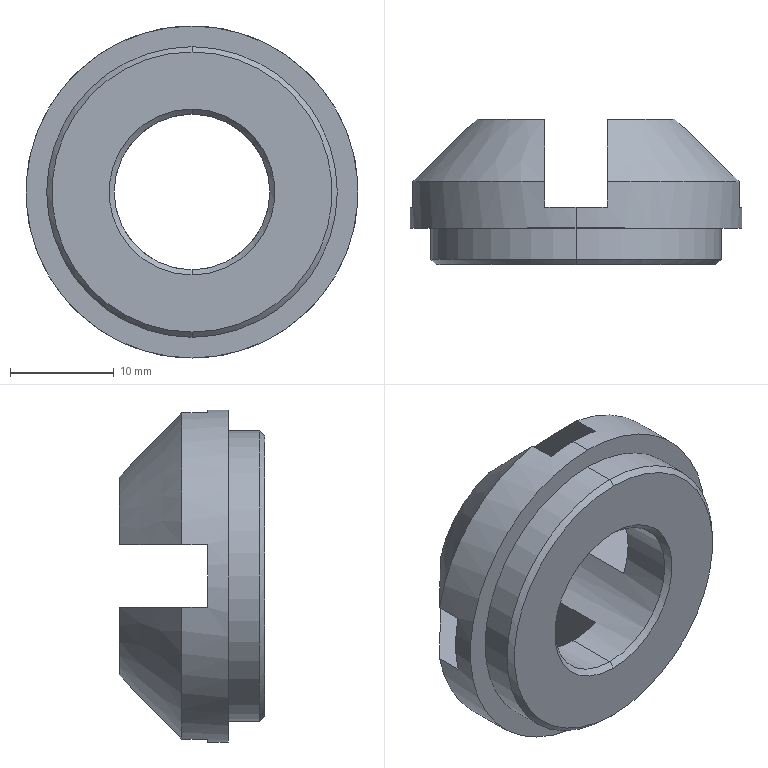Part | SolidWorks | features Chamfer 2, ICE 2, CirPattern 1, Revolution 1 | 1 solid | 32 faces | box 32 x 14 x 32 mm | volume 5204 mm3 | plane 18 | cone 8 | cylinder 6 | commonest cylinder face diameters 15 x2 28 x2 32 x2
STEP:
#1=CARTESIAN_POINT('',(0.,0.5,7.5));
#2=VERTEX_POINT('',#1);
#3=CARTESIAN_POINT('',(0.,0.5,-7.5));
#4=VERTEX_POINT('',#3);
#5=CARTESIAN_POINT('',(0.,0.5,0.));
#6=DIRECTION('',(0.,-1.,0.));
#7=DIRECTION('',(0.,0.,1.));
#8=AXIS2_PLACEMENT_3D('',#5,#6,#7);
#9=CIRCLE('',#8,7.5);
#10=EDGE_CURVE('',#2,#4,#9,.T.);
#11=ORIENTED_EDGE('',*,*,#10,.F.);
#12=CARTESIAN_POINT('',(0.,0.,8.));
#13=VERTEX_POINT('',#12);
#14=CARTESIAN_POINT('',(0.,0.,8.));
#15=DIRECTION('',(0.,-0.7071,0.7071));
#16=VECTOR('',#15,1000.);
#17=LINE('',#14,#16);
#18=EDGE_CURVE('',#2,#13,#17,.T.);
#19=ORIENTED_EDGE('',*,*,#18,.T.);
#20=CARTESIAN_POINT('',(0.,0.,-8.));
#21=VERTEX_POINT('',#20);
#22=CARTESIAN_POINT('',(0.,0.,0.));
#23=DIRECTION('',(0.,1.,0.));
#24=DIRECTION('',(0.,0.,1.));
#25=AXIS2_PLACEMENT_3D('',#22,#23,#24);
#26=CIRCLE('',#25,8.);
#27=EDGE_CURVE('',#21,#13,#26,.T.);
#28=ORIENTED_EDGE('',*,*,#27,.F.);
#29=CARTESIAN_POINT('',(0.,0.,-8.));
#30=DIRECTION('',(0.,-0.7071,-0.7071));
#31=VECTOR('',#30,1000.);
#32=LINE('',#29,#31);
#33=EDGE_CURVE('',#4,#21,#32,.T.);
#34=ORIENTED_EDGE('',*,*,#33,.F.);
#35=EDGE_LOOP('',(#11,#19,#28,#34));
#36=FACE_OUTER_BOUND('',#35,.T.);
#37=CARTESIAN_POINT('',(0.,0.,0.));
#38=DIRECTION('',(0.,-1.,0.));
#39=DIRECTION('',(0.,0.,-1.));
#40=AXIS2_PLACEMENT_3D('',#37,#38,#39);
#41=CONICAL_SURFACE('',#40,8.,0.7854);
#42=ADVANCED_FACE('',(#36),#41,.F.);
#43=CARTESIAN_POINT('',(0.,0.,-13.5));
#44=VERTEX_POINT('',#43);
#45=CARTESIAN_POINT('',(0.,0.,13.5));
#46=VERTEX_POINT('',#45);
#47=CARTESIAN_POINT('',(0.,0.,0.));
#48=DIRECTION('',(0.,-1.,0.));
#49=DIRECTION('',(0.,0.,1.));
#50=AXIS2_PLACEMENT_3D('',#47,#48,#49);
#51=CIRCLE('',#50,13.5);
#52=EDGE_CURVE('',#44,#46,#51,.T.);
#53=ORIENTED_EDGE('',*,*,#52,.F.);
#54=CARTESIAN_POINT('',(0.,0.5,-14.));
#55=VERTEX_POINT('',#54);
#56=CARTESIAN_POINT('',(0.,0.,-13.5));
#57=DIRECTION('',(0.,0.7071,-0.7071));
#58=VECTOR('',#57,1000.);
#59=LINE('',#56,#58);
#60=EDGE_CURVE('',#44,#55,#59,.T.);
#61=ORIENTED_EDGE('',*,*,#60,.T.);
#62=CARTESIAN_POINT('',(0.,0.5,14.));
#63=VERTEX_POINT('',#62);
#64=CARTESIAN_POINT('',(0.,0.5,0.));
#65=DIRECTION('',(0.,1.,0.));
#66=DIRECTION('',(0.,0.,1.));
#67=AXIS2_PLACEMENT_3D('',#64,#65,#66);
#68=CIRCLE('',#67,14.);
#69=EDGE_CURVE('',#63,#55,#68,.T.);
#70=ORIENTED_EDGE('',*,*,#69,.F.);
#71=CARTESIAN_POINT('',(0.,0.,13.5));
#72=DIRECTION('',(0.,0.7071,0.7071));
#73=VECTOR('',#72,1000.);
#74=LINE('',#71,#73);
#75=EDGE_CURVE('',#46,#63,#74,.T.);
#76=ORIENTED_EDGE('',*,*,#75,.F.);
#77=EDGE_LOOP('',(#53,#61,#70,#76));
#78=FACE_OUTER_BOUND('',#77,.T.);
#79=CARTESIAN_POINT('',(0.,0.,0.));
#80=DIRECTION('',(0.,1.,0.));
#81=DIRECTION('',(0.,0.,1.));
#82=AXIS2_PLACEMENT_3D('',#79,#80,#81);
#83=CONICAL_SURFACE('',#82,13.5,0.7854);
#84=ADVANCED_FACE('',(#78),#83,.T.);
#85=ORIENTED_EDGE('',*,*,#10,.T.);
#86=CARTESIAN_POINT('',(0.,5.5,-7.5));
#87=VERTEX_POINT('',#86);
#88=CARTESIAN_POINT('',(0.,-17.,-7.5));
#89=DIRECTION('',(0.,1.,0.));
#90=VECTOR('',#89,1000.);
#91=LINE('',#88,#90);
#92=EDGE_CURVE('',#4,#87,#91,.T.);
#93=ORIENTED_EDGE('',*,*,#92,.T.);
#94=CARTESIAN_POINT('',(-3.,5.5,-6.874));
#95=VERTEX_POINT('',#94);
#96=CARTESIAN_POINT('',(0.,5.5,0.));
#97=DIRECTION('',(0.,-1.,0.));
#98=DIRECTION('',(0.,0.,1.));
#99=AXIS2_PLACEMENT_3D('',#96,#97,#98);
#100=CIRCLE('',#99,7.5);
#101=EDGE_CURVE('',#95,#87,#100,.T.);
#102=ORIENTED_EDGE('',*,*,#101,.F.);
#103=CARTESIAN_POINT('',(-3.,14.,-6.874));
#104=VERTEX_POINT('',#103);
#105=CARTESIAN_POINT('',(-3.,-17.,-6.874));
#106=DIRECTION('',(0.,1.,0.));
#107=VECTOR('',#106,1000.);
#108=LINE('',#105,#107);
#109=EDGE_CURVE('',#95,#104,#108,.T.);
#110=ORIENTED_EDGE('',*,*,#109,.T.);
#111=CARTESIAN_POINT('',(-6.874,14.,-3.));
#112=VERTEX_POINT('',#111);
#113=CARTESIAN_POINT('',(0.,14.,0.));
#114=DIRECTION('',(0.,1.,0.));
#115=DIRECTION('',(0.,0.,1.));
#116=AXIS2_PLACEMENT_3D('',#113,#114,#115);
#117=CIRCLE('',#116,7.5);
#118=EDGE_CURVE('',#104,#112,#117,.T.);
#119=ORIENTED_EDGE('',*,*,#118,.T.);
#120=CARTESIAN_POINT('',(-6.874,5.5,-3.));
#121=VERTEX_POINT('',#120);
#122=CARTESIAN_POINT('',(-6.874,-17.,-3.));
#123=DIRECTION('',(0.,-1.,0.));
#124=VECTOR('',#123,1000.);
#125=LINE('',#122,#124);
#126=EDGE_CURVE('',#112,#121,#125,.T.);
#127=ORIENTED_EDGE('',*,*,#126,.T.);
#128=CARTESIAN_POINT('',(-6.874,5.5,3.));
#129=VERTEX_POINT('',#128);
#130=CARTESIAN_POINT('',(0.,5.5,0.));
#131=DIRECTION('',(0.,-1.,0.));
#132=DIRECTION('',(0.,0.,1.));
#133=AXIS2_PLACEMENT_3D('',#130,#131,#132);
#134=CIRCLE('',#133,7.5);
#135=EDGE_CURVE('',#129,#121,#134,.T.);
#136=ORIENTED_EDGE('',*,*,#135,.F.);
#137=CARTESIAN_POINT('',(-6.874,14.,3.));
#138=VERTEX_POINT('',#137);
#139=CARTESIAN_POINT('',(-6.874,-17.,3.));
#140=DIRECTION('',(0.,1.,0.));
#141=VECTOR('',#140,1000.);
#142=LINE('',#139,#141);
#143=EDGE_CURVE('',#129,#138,#142,.T.);
#144=ORIENTED_EDGE('',*,*,#143,.T.);
#145=CARTESIAN_POINT('',(-3.,14.,6.874));
#146=VERTEX_POINT('',#145);
#147=CARTESIAN_POINT('',(0.,14.,0.));
#148=DIRECTION('',(0.,1.,0.));
#149=DIRECTION('',(0.,0.,1.));
#150=AXIS2_PLACEMENT_3D('',#147,#148,#149);
#151=CIRCLE('',#150,7.5);
#152=EDGE_CURVE('',#138,#146,#151,.T.);
#153=ORIENTED_EDGE('',*,*,#152,.T.);
#154=CARTESIAN_POINT('',(-3.,5.5,6.874));
#155=VERTEX_POINT('',#154);
#156=CARTESIAN_POINT('',(-3.,-17.,6.874));
#157=DIRECTION('',(0.,-1.,0.));
#158=VECTOR('',#157,1000.);
#159=LINE('',#156,#158);
#160=EDGE_CURVE('',#146,#155,#159,.T.);
#161=ORIENTED_EDGE('',*,*,#160,.T.);
#162=CARTESIAN_POINT('',(0.,5.5,7.5));
#163=VERTEX_POINT('',#162);
#164=CARTESIAN_POINT('',(0.,5.5,0.));
#165=DIRECTION('',(0.,-1.,0.));
#166=DIRECTION('',(0.,0.,1.));
#167=AXIS2_PLACEMENT_3D('',#164,#165,#166);
#168=CIRCLE('',#167,7.5);
#169=EDGE_CURVE('',#163,#155,#168,.T.);
#170=ORIENTED_EDGE('',*,*,#169,.F.);
#171=CARTESIAN_POINT('',(0.,-17.,7.5));
#172=DIRECTION('',(0.,1.,0.));
#173=VECTOR('',#172,1000.);
#174=LINE('',#171,#173);
#175=EDGE_CURVE('',#2,#163,#174,.T.);
#176=ORIENTED_EDGE('',*,*,#175,.F.);
#177=EDGE_LOOP('',(#85,#93,#102,#110,#119,#127,#136,#144,#153,#161,#170,#176));
#178=FACE_OUTER_BOUND('',#177,.T.);
#179=CARTESIAN_POINT('',(0.,-17.,0.));
#180=DIRECTION('',(0.,1.,0.));
#181=DIRECTION('',(0.,0.,1.));
#182=AXIS2_PLACEMENT_3D('',#179,#180,#181);
#183=CYLINDRICAL_SURFACE('',#182,7.5);
#184=ADVANCED_FACE('',(#178),#183,.F.);
#185=CARTESIAN_POINT('',(0.,5.5,16.));
#186=VERTEX_POINT('',#185);
#187=CARTESIAN_POINT('',(3.,5.5,15.716));
#188=VERTEX_POINT('',#187);
#189=CARTESIAN_POINT('',(0.,5.5,0.));
#190=DIRECTION('',(0.,1.,0.));
#191=DIRECTION('',(0.,0.,1.));
#192=AXIS2_PLACEMENT_3D('',#189,#190,#191);
#193=CIRCLE('',#192,16.);
#194=EDGE_CURVE('',#186,#188,#193,.T.);
#195=ORIENTED_EDGE('',*,*,#194,.F.);
#196=CARTESIAN_POINT('',(0.,3.5,16.));
#197=VERTEX_POINT('',#196);
#198=CARTESIAN_POINT('',(0.,0.,16.));
#199=DIRECTION('',(0.,-1.,0.));
#200=VECTOR('',#199,1000.);
#201=LINE('',#198,#200);
#202=EDGE_CURVE('',#186,#197,#201,.T.);
#203=ORIENTED_EDGE('',*,*,#202,.T.);
#204=CARTESIAN_POINT('',(0.,3.5,-16.));
#205=VERTEX_POINT('',#204);
#206=CARTESIAN_POINT('',(0.,3.5,0.));
#207=DIRECTION('',(0.,-1.,0.));
#208=DIRECTION('',(0.,0.,-1.));
#209=AXIS2_PLACEMENT_3D('',#206,#207,#208);
#210=CIRCLE('',#209,16.);
#211=EDGE_CURVE('',#205,#197,#210,.T.);
#212=ORIENTED_EDGE('',*,*,#211,.F.);
#213=CARTESIAN_POINT('',(0.,5.5,-16.));
#214=VERTEX_POINT('',#213);
#215=CARTESIAN_POINT('',(0.,0.,-16.));
#216=DIRECTION('',(0.,-1.,0.));
#217=VECTOR('',#216,1000.);
#218=LINE('',#215,#217);
#219=EDGE_CURVE('',#214,#205,#218,.T.);
#220=ORIENTED_EDGE('',*,*,#219,.F.);
#221=CARTESIAN_POINT('',(3.,5.5,-15.716));
#222=VERTEX_POINT('',#221);
#223=CARTESIAN_POINT('',(0.,5.5,0.));
#224=DIRECTION('',(0.,1.,0.));
#225=DIRECTION('',(0.,0.,1.));
#226=AXIS2_PLACEMENT_3D('',#223,#224,#225);
#227=CIRCLE('',#226,16.);
#228=EDGE_CURVE('',#222,#214,#227,.T.);
#229=ORIENTED_EDGE('',*,*,#228,.F.);
#230=CARTESIAN_POINT('',(3.,8.,-15.716));
#231=VERTEX_POINT('',#230);
#232=CARTESIAN_POINT('',(3.,0.,-15.716));
#233=DIRECTION('',(0.,1.,0.));
#234=VECTOR('',#233,1000.);
#235=LINE('',#232,#234);
#236=EDGE_CURVE('',#222,#231,#235,.T.);
#237=ORIENTED_EDGE('',*,*,#236,.T.);
#238=CARTESIAN_POINT('',(15.716,8.,-3.));
#239=VERTEX_POINT('',#238);
#240=CARTESIAN_POINT('',(0.,8.,0.));
#241=DIRECTION('',(0.,-1.,0.));
#242=DIRECTION('',(0.,0.,-1.));
#243=AXIS2_PLACEMENT_3D('',#240,#241,#242);
#244=CIRCLE('',#243,16.);
#245=EDGE_CURVE('',#231,#239,#244,.T.);
#246=ORIENTED_EDGE('',*,*,#245,.T.);
#247=CARTESIAN_POINT('',(15.716,5.5,-3.));
#248=VERTEX_POINT('',#247);
#249=CARTESIAN_POINT('',(15.716,0.,-3.));
#250=DIRECTION('',(0.,-1.,0.));
#251=VECTOR('',#250,1000.);
#252=LINE('',#249,#251);
#253=EDGE_CURVE('',#239,#248,#252,.T.);
#254=ORIENTED_EDGE('',*,*,#253,.T.);
#255=CARTESIAN_POINT('',(15.716,5.5,3.));
#256=VERTEX_POINT('',#255);
#257=CARTESIAN_POINT('',(0.,5.5,0.));
#258=DIRECTION('',(0.,1.,0.));
#259=DIRECTION('',(0.,0.,1.));
#260=AXIS2_PLACEMENT_3D('',#257,#258,#259);
#261=CIRCLE('',#260,16.);
#262=EDGE_CURVE('',#256,#248,#261,.T.);
#263=ORIENTED_EDGE('',*,*,#262,.F.);
#264=CARTESIAN_POINT('',(15.716,8.,3.));
#265=VERTEX_POINT('',#264);
#266=CARTESIAN_POINT('',(15.716,0.,3.));
#267=DIRECTION('',(0.,1.,0.));
#268=VECTOR('',#267,1000.);
#269=LINE('',#266,#268);
#270=EDGE_CURVE('',#256,#265,#269,.T.);
#271=ORIENTED_EDGE('',*,*,#270,.T.);
#272=CARTESIAN_POINT('',(3.,8.,15.716));
#273=VERTEX_POINT('',#272);
#274=CARTESIAN_POINT('',(0.,8.,0.));
#275=DIRECTION('',(0.,-1.,0.));
#276=DIRECTION('',(0.,0.,-1.));
#277=AXIS2_PLACEMENT_3D('',#274,#275,#276);
#278=CIRCLE('',#277,16.);
#279=EDGE_CURVE('',#265,#273,#278,.T.);
#280=ORIENTED_EDGE('',*,*,#279,.T.);
#281=CARTESIAN_POINT('',(3.,0.,15.716));
#282=DIRECTION('',(0.,-1.,0.));
#283=VECTOR('',#282,1000.);
#284=LINE('',#281,#283);
#285=EDGE_CURVE('',#273,#188,#284,.T.);
#286=ORIENTED_EDGE('',*,*,#285,.T.);
#287=EDGE_LOOP('',(#195,#203,#212,#220,#229,#237,#246,#254,#263,#271,#280,#286));
#288=FACE_OUTER_BOUND('',#287,.T.);
#289=CARTESIAN_POINT('',(0.,0.,0.));
#290=DIRECTION('',(0.,-1.,0.));
#291=DIRECTION('',(0.,0.,-1.));
#292=AXIS2_PLACEMENT_3D('',#289,#290,#291);
#293=CYLINDRICAL_SURFACE('',#292,16.);
#294=ADVANCED_FACE('',(#288),#293,.T.);
#295=CARTESIAN_POINT('',(0.,3.5,-14.));
#296=VERTEX_POINT('',#295);
#297=CARTESIAN_POINT('',(0.,3.5,14.));
#298=VERTEX_POINT('',#297);
#299=CARTESIAN_POINT('',(0.,3.5,0.));
#300=DIRECTION('',(0.,-1.,0.));
#301=DIRECTION('',(0.,0.,-1.));
#302=AXIS2_PLACEMENT_3D('',#299,#300,#301);
#303=CIRCLE('',#302,14.);
#304=EDGE_CURVE('',#296,#298,#303,.T.);
#305=ORIENTED_EDGE('',*,*,#304,.T.);
#306=CARTESIAN_POINT('',(0.,0.,14.));
#307=DIRECTION('',(0.,-1.,0.));
#308=VECTOR('',#307,1000.);
#309=LINE('',#306,#308);
#310=EDGE_CURVE('',#298,#63,#309,.T.);
#311=ORIENTED_EDGE('',*,*,#310,.T.);
#312=ORIENTED_EDGE('',*,*,#69,.T.);
#313=CARTESIAN_POINT('',(0.,0.,-14.));
#314=DIRECTION('',(0.,-1.,0.));
#315=VECTOR('',#314,1000.);
#316=LINE('',#313,#315);
#317=EDGE_CURVE('',#296,#55,#316,.T.);
#318=ORIENTED_EDGE('',*,*,#317,.F.);
#319=EDGE_LOOP('',(#305,#311,#312,#318));
#320=FACE_OUTER_BOUND('',#319,.T.);
#321=CARTESIAN_POINT('',(0.,0.,0.));
#322=DIRECTION('',(0.,-1.,0.));
#323=DIRECTION('',(0.,0.,-1.));
#324=AXIS2_PLACEMENT_3D('',#321,#322,#323);
#325=CYLINDRICAL_SURFACE('',#324,14.);
#326=ADVANCED_FACE('',(#320),#325,.T.);
#327=CARTESIAN_POINT('',(9.539,14.,3.));
#328=VERTEX_POINT('',#327);
#329=CARTESIAN_POINT('',(3.,14.,9.539));
#330=VERTEX_POINT('',#329);
#331=CARTESIAN_POINT('',(0.,14.,0.));
#332=DIRECTION('',(0.,-1.,0.));
#333=DIRECTION('',(0.,0.,-1.));
#334=AXIS2_PLACEMENT_3D('',#331,#332,#333);
#335=CIRCLE('',#334,10.);
#336=EDGE_CURVE('',#328,#330,#335,.T.);
#337=ORIENTED_EDGE('',*,*,#336,.T.);
#338=CARTESIAN_POINT('',(3.,14.,9.539));
#339=CARTESIAN_POINT('',(3.,12.019,11.616));
#340=CARTESIAN_POINT('',(3.,10.012,13.668));
#341=CARTESIAN_POINT('',(3.,8.,15.716));
#342=B_SPLINE_CURVE_WITH_KNOTS('',3,(#338,#339,#340,#341),.UNSPECIFIED.,.F.,.F.,(4,4),(0.01205,0.02069),.UNSPECIFIED.);
#343=EDGE_CURVE('',#330,#273,#342,.T.);
#344=ORIENTED_EDGE('',*,*,#343,.T.);
#345=ORIENTED_EDGE('',*,*,#279,.F.);
#346=CARTESIAN_POINT('',(15.716,8.,3.));
#347=CARTESIAN_POINT('',(13.668,10.012,3.));
#348=CARTESIAN_POINT('',(11.616,12.019,3.));
#349=CARTESIAN_POINT('',(9.539,14.,3.));
#350=B_SPLINE_CURVE_WITH_KNOTS('',3,(#346,#347,#348,#349),.UNSPECIFIED.,.F.,.F.,(4,4),(0.000000998,0.008605),.UNSPECIFIED.);
#351=EDGE_CURVE('',#265,#328,#350,.T.);
#352=ORIENTED_EDGE('',*,*,#351,.T.);
#353=EDGE_LOOP('',(#337,#344,#345,#352));
#354=FACE_OUTER_BOUND('',#353,.T.);
#355=CARTESIAN_POINT('',(0.,14.,0.));
#356=DIRECTION('',(0.,-1.,0.));
#357=DIRECTION('',(0.,0.,-1.));
#358=AXIS2_PLACEMENT_3D('',#355,#356,#357);
#359=CONICAL_SURFACE('',#358,10.,0.7854);
#360=ADVANCED_FACE('',(#354),#359,.T.);
#361=CARTESIAN_POINT('',(3.,14.,6.874));
#362=VERTEX_POINT('',#361);
#363=CARTESIAN_POINT('',(6.874,14.,3.));
#364=VERTEX_POINT('',#363);
#365=CARTESIAN_POINT('',(0.,14.,0.));
#366=DIRECTION('',(0.,1.,0.));
#367=DIRECTION('',(0.,0.,1.));
#368=AXIS2_PLACEMENT_3D('',#365,#366,#367);
#369=CIRCLE('',#368,7.5);
#370=EDGE_CURVE('',#362,#364,#369,.T.);
#371=ORIENTED_EDGE('',*,*,#370,.F.);
#372=CARTESIAN_POINT('',(3.,14.,20.34));
#373=DIRECTION('',(0.,0.,-1.));
#374=VECTOR('',#373,1000.);
#375=LINE('',#372,#374);
#376=EDGE_CURVE('',#330,#362,#375,.T.);
#377=ORIENTED_EDGE('',*,*,#376,.F.);
#378=ORIENTED_EDGE('',*,*,#336,.F.);
#379=CARTESIAN_POINT('',(-20.34,14.,3.));
#380=DIRECTION('',(1.,0.,0.));
#381=VECTOR('',#380,1000.);
#382=LINE('',#379,#381);
#383=EDGE_CURVE('',#364,#328,#382,.T.);
#384=ORIENTED_EDGE('',*,*,#383,.F.);
#385=EDGE_LOOP('',(#371,#377,#378,#384));
#386=FACE_OUTER_BOUND('',#385,.T.);
#387=CARTESIAN_POINT('',(-10.,14.,0.));
#388=DIRECTION('',(0.,-1.,0.));
#389=DIRECTION('',(0.,0.,-1.));
#390=AXIS2_PLACEMENT_3D('',#387,#388,#389);
#391=PLANE('',#390);
#392=ADVANCED_FACE('',(#386),#391,.F.);
#393=ORIENTED_EDGE('',*,*,#245,.F.);
#394=CARTESIAN_POINT('',(3.,14.,-9.539));
#395=VERTEX_POINT('',#394);
#396=CARTESIAN_POINT('',(3.,8.,-15.716));
#397=CARTESIAN_POINT('',(3.,10.011,-13.668));
#398=CARTESIAN_POINT('',(3.,12.019,-11.616));
#399=CARTESIAN_POINT('',(3.,14.,-9.539));
#400=B_SPLINE_CURVE_WITH_KNOTS('',3,(#396,#397,#398,#399),.UNSPECIFIED.,.F.,.F.,(4,4),(0.000000999,0.008612),.UNSPECIFIED.);
#401=EDGE_CURVE('',#231,#395,#400,.T.);
#402=ORIENTED_EDGE('',*,*,#401,.T.);
#403=CARTESIAN_POINT('',(9.539,14.,-3.));
#404=VERTEX_POINT('',#403);
#405=CARTESIAN_POINT('',(0.,14.,0.));
#406=DIRECTION('',(0.,-1.,0.));
#407=DIRECTION('',(0.,0.,-1.));
#408=AXIS2_PLACEMENT_3D('',#405,#406,#407);
#409=CIRCLE('',#408,10.);
#410=EDGE_CURVE('',#395,#404,#409,.T.);
#411=ORIENTED_EDGE('',*,*,#410,.T.);
#412=CARTESIAN_POINT('',(9.539,14.,-3.));
#413=CARTESIAN_POINT('',(11.616,12.019,-3.));
#414=CARTESIAN_POINT('',(13.668,10.012,-3.));
#415=CARTESIAN_POINT('',(15.716,8.,-3.));
#416=B_SPLINE_CURVE_WITH_KNOTS('',3,(#412,#413,#414,#415),.UNSPECIFIED.,.F.,.F.,(4,4),(0.03228,0.0407),.UNSPECIFIED.);
#417=EDGE_CURVE('',#404,#239,#416,.T.);
#418=ORIENTED_EDGE('',*,*,#417,.T.);
#419=EDGE_LOOP('',(#393,#402,#411,#418));
#420=FACE_OUTER_BOUND('',#419,.T.);
#421=CARTESIAN_POINT('',(0.,14.,0.));
#422=DIRECTION('',(0.,-1.,0.));
#423=DIRECTION('',(0.,0.,-1.));
#424=AXIS2_PLACEMENT_3D('',#421,#422,#423);
#425=CONICAL_SURFACE('',#424,10.,0.7854);
#426=ADVANCED_FACE('',(#420),#425,.T.);
#427=ORIENTED_EDGE('',*,*,#410,.F.);
#428=CARTESIAN_POINT('',(3.,14.,-6.874));
#429=VERTEX_POINT('',#428);
#430=CARTESIAN_POINT('',(3.,14.,20.34));
#431=DIRECTION('',(0.,0.,-1.));
#432=VECTOR('',#431,1000.);
#433=LINE('',#430,#432);
#434=EDGE_CURVE('',#429,#395,#433,.T.);
#435=ORIENTED_EDGE('',*,*,#434,.F.);
#436=CARTESIAN_POINT('',(6.874,14.,-3.));
#437=VERTEX_POINT('',#436);
#438=CARTESIAN_POINT('',(0.,14.,0.));
#439=DIRECTION('',(0.,1.,0.));
#440=DIRECTION('',(0.,0.,1.));
#441=AXIS2_PLACEMENT_3D('',#438,#439,#440);
#442=CIRCLE('',#441,7.5);
#443=EDGE_CURVE('',#437,#429,#442,.T.);
#444=ORIENTED_EDGE('',*,*,#443,.F.);
#445=CARTESIAN_POINT('',(-20.34,14.,-3.));
#446=DIRECTION('',(-1.,0.,0.));
#447=VECTOR('',#446,1000.);
#448=LINE('',#445,#447);
#449=EDGE_CURVE('',#404,#437,#448,.T.);
#450=ORIENTED_EDGE('',*,*,#449,.F.);
#451=EDGE_LOOP('',(#427,#435,#444,#450));
#452=FACE_OUTER_BOUND('',#451,.T.);
#453=CARTESIAN_POINT('',(-10.,14.,0.));
#454=DIRECTION('',(0.,-1.,0.));
#455=DIRECTION('',(0.,0.,-1.));
#456=AXIS2_PLACEMENT_3D('',#453,#454,#455);
#457=PLANE('',#456);
#458=ADVANCED_FACE('',(#452),#457,.F.);
#459=CARTESIAN_POINT('',(-3.,8.,15.716));
#460=VERTEX_POINT('',#459);
#461=CARTESIAN_POINT('',(-15.716,8.,3.));
#462=VERTEX_POINT('',#461);
#463=CARTESIAN_POINT('',(0.,8.,0.));
#464=DIRECTION('',(0.,-1.,0.));
#465=DIRECTION('',(0.,0.,-1.));
#466=AXIS2_PLACEMENT_3D('',#463,#464,#465);
#467=CIRCLE('',#466,16.);
#468=EDGE_CURVE('',#460,#462,#467,.T.);
#469=ORIENTED_EDGE('',*,*,#468,.F.);
#470=CARTESIAN_POINT('',(-3.,14.,9.539));
#471=VERTEX_POINT('',#470);
#472=CARTESIAN_POINT('',(-3.,8.,15.716));
#473=CARTESIAN_POINT('',(-3.,10.011,13.668));
#474=CARTESIAN_POINT('',(-3.,12.019,11.616));
#475=CARTESIAN_POINT('',(-3.,14.,9.539));
#476=B_SPLINE_CURVE_WITH_KNOTS('',3,(#472,#473,#474,#475),.UNSPECIFIED.,.F.,.F.,(4,4),(0.000000999,0.008612),.UNSPECIFIED.);
#477=EDGE_CURVE('',#460,#471,#476,.T.);
#478=ORIENTED_EDGE('',*,*,#477,.T.);
#479=CARTESIAN_POINT('',(-9.539,14.,3.));
#480=VERTEX_POINT('',#479);
#481=CARTESIAN_POINT('',(0.,14.,0.));
#482=DIRECTION('',(0.,-1.,0.));
#483=DIRECTION('',(0.,0.,-1.));
#484=AXIS2_PLACEMENT_3D('',#481,#482,#483);
#485=CIRCLE('',#484,10.);
#486=EDGE_CURVE('',#471,#480,#485,.T.);
#487=ORIENTED_EDGE('',*,*,#486,.T.);
#488=CARTESIAN_POINT('',(-9.539,14.,3.));
#489=CARTESIAN_POINT('',(-11.616,12.019,3.));
#490=CARTESIAN_POINT('',(-13.668,10.012,3.));
#491=CARTESIAN_POINT('',(-15.716,8.,3.));
#492=B_SPLINE_CURVE_WITH_KNOTS('',3,(#488,#489,#490,#491),.UNSPECIFIED.,.F.,.F.,(4,4),(0.03228,0.0407),.UNSPECIFIED.);
#493=EDGE_CURVE('',#480,#462,#492,.T.);
#494=ORIENTED_EDGE('',*,*,#493,.T.);
#495=EDGE_LOOP('',(#469,#478,#487,#494));
#496=FACE_OUTER_BOUND('',#495,.T.);
#497=CARTESIAN_POINT('',(0.,14.,0.));
#498=DIRECTION('',(0.,-1.,0.));
#499=DIRECTION('',(0.,0.,-1.));
#500=AXIS2_PLACEMENT_3D('',#497,#498,#499);
#501=CONICAL_SURFACE('',#500,10.,0.7854);
#502=ADVANCED_FACE('',(#496),#501,.T.);
#503=ORIENTED_EDGE('',*,*,#486,.F.);
#504=CARTESIAN_POINT('',(-3.,14.,20.34));
#505=DIRECTION('',(0.,0.,1.));
#506=VECTOR('',#505,1000.);
#507=LINE('',#504,#506);
#508=EDGE_CURVE('',#146,#471,#507,.T.);
#509=ORIENTED_EDGE('',*,*,#508,.F.);
#510=ORIENTED_EDGE('',*,*,#152,.F.);
#511=CARTESIAN_POINT('',(-20.34,14.,3.));
#512=DIRECTION('',(1.,0.,0.));
#513=VECTOR('',#512,1000.);
#514=LINE('',#511,#513);
#515=EDGE_CURVE('',#480,#138,#514,.T.);
#516=ORIENTED_EDGE('',*,*,#515,.F.);
#517=EDGE_LOOP('',(#503,#509,#510,#516));
#518=FACE_OUTER_BOUND('',#517,.T.);
#519=CARTESIAN_POINT('',(-10.,14.,0.));
#520=DIRECTION('',(0.,-1.,0.));
#521=DIRECTION('',(0.,0.,-1.));
#522=AXIS2_PLACEMENT_3D('',#519,#520,#521);
#523=PLANE('',#522);
#524=ADVANCED_FACE('',(#518),#523,.F.);
#525=ORIENTED_EDGE('',*,*,#27,.T.);
#526=CARTESIAN_POINT('',(0.,0.,0.));
#527=DIRECTION('',(0.,1.,0.));
#528=DIRECTION('',(0.,0.,1.));
#529=AXIS2_PLACEMENT_3D('',#526,#527,#528);
#530=CIRCLE('',#529,8.);
#531=EDGE_CURVE('',#13,#21,#530,.T.);
#532=ORIENTED_EDGE('',*,*,#531,.T.);
#533=EDGE_LOOP('',(#525,#532));
#534=FACE_BOUND('',#533,.T.);
#535=CARTESIAN_POINT('',(0.,0.,0.));
#536=DIRECTION('',(0.,-1.,0.));
#537=DIRECTION('',(0.,0.,1.));
#538=AXIS2_PLACEMENT_3D('',#535,#536,#537);
#539=CIRCLE('',#538,13.5);
#540=EDGE_CURVE('',#46,#44,#539,.T.);
#541=ORIENTED_EDGE('',*,*,#540,.T.);
#542=ORIENTED_EDGE('',*,*,#52,.T.);
#543=EDGE_LOOP('',(#541,#542));
#544=FACE_OUTER_BOUND('',#543,.T.);
#545=CARTESIAN_POINT('',(0.,0.,0.));
#546=DIRECTION('',(0.,1.,0.));
#547=DIRECTION('',(0.,0.,1.));
#548=AXIS2_PLACEMENT_3D('',#545,#546,#547);
#549=PLANE('',#548);
#550=ADVANCED_FACE('',(#534,#544),#549,.F.);
#551=ORIENTED_EDGE('',*,*,#310,.F.);
#552=CARTESIAN_POINT('',(0.,3.5,0.));
#553=DIRECTION('',(0.,-1.,0.));
#554=DIRECTION('',(0.,0.,-1.));
#555=AXIS2_PLACEMENT_3D('',#552,#553,#554);
#556=CIRCLE('',#555,14.);
#557=EDGE_CURVE('',#298,#296,#556,.T.);
#558=ORIENTED_EDGE('',*,*,#557,.T.);
#559=ORIENTED_EDGE('',*,*,#317,.T.);
#560=CARTESIAN_POINT('',(0.,0.5,0.));
#561=DIRECTION('',(0.,1.,0.));
#562=DIRECTION('',(0.,0.,1.));
#563=AXIS2_PLACEMENT_3D('',#560,#561,#562);
#564=CIRCLE('',#563,14.);
#565=EDGE_CURVE('',#55,#63,#564,.T.);
#566=ORIENTED_EDGE('',*,*,#565,.T.);
#567=EDGE_LOOP('',(#551,#558,#559,#566));
#568=FACE_OUTER_BOUND('',#567,.T.);
#569=CARTESIAN_POINT('',(0.,0.,0.));
#570=DIRECTION('',(0.,-1.,0.));
#571=DIRECTION('',(0.,0.,-1.));
#572=AXIS2_PLACEMENT_3D('',#569,#570,#571);
#573=CYLINDRICAL_SURFACE('',#572,14.);
#574=ADVANCED_FACE('',(#568),#573,.T.);
#575=ORIENTED_EDGE('',*,*,#304,.F.);
#576=ORIENTED_EDGE('',*,*,#557,.F.);
#577=EDGE_LOOP('',(#575,#576));
#578=FACE_BOUND('',#577,.T.);
#579=ORIENTED_EDGE('',*,*,#211,.T.);
#580=CARTESIAN_POINT('',(0.,3.5,0.));
#581=DIRECTION('',(0.,-1.,0.));
#582=DIRECTION('',(0.,0.,-1.));
#583=AXIS2_PLACEMENT_3D('',#580,#581,#582);
#584=CIRCLE('',#583,16.);
#585=EDGE_CURVE('',#197,#205,#584,.T.);
#586=ORIENTED_EDGE('',*,*,#585,.T.);
#587=EDGE_LOOP('',(#579,#586));
#588=FACE_OUTER_BOUND('',#587,.T.);
#589=CARTESIAN_POINT('',(-14.,3.5,0.));
#590=DIRECTION('',(0.,1.,0.));
#591=DIRECTION('',(0.,0.,1.));
#592=AXIS2_PLACEMENT_3D('',#589,#590,#591);
#593=PLANE('',#592);
#594=ADVANCED_FACE('',(#578,#588),#593,.F.);
#595=ORIENTED_EDGE('',*,*,#202,.F.);
#596=CARTESIAN_POINT('',(-3.,5.5,15.716));
#597=VERTEX_POINT('',#596);
#598=CARTESIAN_POINT('',(0.,5.5,0.));
#599=DIRECTION('',(0.,1.,0.));
#600=DIRECTION('',(0.,0.,1.));
#601=AXIS2_PLACEMENT_3D('',#598,#599,#600);
#602=CIRCLE('',#601,16.);
#603=EDGE_CURVE('',#597,#186,#602,.T.);
#604=ORIENTED_EDGE('',*,*,#603,.F.);
#605=CARTESIAN_POINT('',(-3.,0.,15.716));
#606=DIRECTION('',(0.,1.,0.));
#607=VECTOR('',#606,1000.);
#608=LINE('',#605,#607);
#609=EDGE_CURVE('',#597,#460,#608,.T.);
#610=ORIENTED_EDGE('',*,*,#609,.T.);
#611=ORIENTED_EDGE('',*,*,#468,.T.);
#612=CARTESIAN_POINT('',(-15.716,5.5,3.));
#613=VERTEX_POINT('',#612);
#614=CARTESIAN_POINT('',(-15.716,0.,3.));
#615=DIRECTION('',(0.,-1.,0.));
#616=VECTOR('',#615,1000.);
#617=LINE('',#614,#616);
#618=EDGE_CURVE('',#462,#613,#617,.T.);
#619=ORIENTED_EDGE('',*,*,#618,.T.);
#620=CARTESIAN_POINT('',(-15.716,5.5,-3.));
#621=VERTEX_POINT('',#620);
#622=CARTESIAN_POINT('',(0.,5.5,0.));
#623=DIRECTION('',(0.,1.,0.));
#624=DIRECTION('',(0.,0.,1.));
#625=AXIS2_PLACEMENT_3D('',#622,#623,#624);
#626=CIRCLE('',#625,16.);
#627=EDGE_CURVE('',#621,#613,#626,.T.);
#628=ORIENTED_EDGE('',*,*,#627,.F.);
#629=CARTESIAN_POINT('',(-15.716,8.,-3.));
#630=VERTEX_POINT('',#629);
#631=CARTESIAN_POINT('',(-15.716,0.,-3.));
#632=DIRECTION('',(0.,1.,0.));
#633=VECTOR('',#632,1000.);
#634=LINE('',#631,#633);
#635=EDGE_CURVE('',#621,#630,#634,.T.);
#636=ORIENTED_EDGE('',*,*,#635,.T.);
#637=CARTESIAN_POINT('',(-3.,8.,-15.716));
#638=VERTEX_POINT('',#637);
#639=CARTESIAN_POINT('',(0.,8.,0.));
#640=DIRECTION('',(0.,-1.,0.));
#641=DIRECTION('',(0.,0.,-1.));
#642=AXIS2_PLACEMENT_3D('',#639,#640,#641);
#643=CIRCLE('',#642,16.);
#644=EDGE_CURVE('',#630,#638,#643,.T.);
#645=ORIENTED_EDGE('',*,*,#644,.T.);
#646=CARTESIAN_POINT('',(-3.,5.5,-15.716));
#647=VERTEX_POINT('',#646);
#648=CARTESIAN_POINT('',(-3.,0.,-15.716));
#649=DIRECTION('',(0.,-1.,0.));
#650=VECTOR('',#649,1000.);
#651=LINE('',#648,#650);
#652=EDGE_CURVE('',#638,#647,#651,.T.);
#653=ORIENTED_EDGE('',*,*,#652,.T.);
#654=CARTESIAN_POINT('',(0.,5.5,0.));
#655=DIRECTION('',(0.,1.,0.));
#656=DIRECTION('',(0.,0.,1.));
#657=AXIS2_PLACEMENT_3D('',#654,#655,#656);
#658=CIRCLE('',#657,16.);
#659=EDGE_CURVE('',#214,#647,#658,.T.);
#660=ORIENTED_EDGE('',*,*,#659,.F.);
#661=ORIENTED_EDGE('',*,*,#219,.T.);
#662=ORIENTED_EDGE('',*,*,#585,.F.);
#663=EDGE_LOOP('',(#595,#604,#610,#611,#619,#628,#636,#645,#653,#660,#661,#662));
#664=FACE_OUTER_BOUND('',#663,.T.);
#665=CARTESIAN_POINT('',(0.,0.,0.));
#666=DIRECTION('',(0.,-1.,0.));
#667=DIRECTION('',(0.,0.,-1.));
#668=AXIS2_PLACEMENT_3D('',#665,#666,#667);
#669=CYLINDRICAL_SURFACE('',#668,16.);
#670=ADVANCED_FACE('',(#664),#669,.T.);
#671=CARTESIAN_POINT('',(-9.539,14.,-3.));
#672=VERTEX_POINT('',#671);
#673=CARTESIAN_POINT('',(-3.,14.,-9.539));
#674=VERTEX_POINT('',#673);
#675=CARTESIAN_POINT('',(0.,14.,0.));
#676=DIRECTION('',(0.,-1.,0.));
#677=DIRECTION('',(0.,0.,-1.));
#678=AXIS2_PLACEMENT_3D('',#675,#676,#677);
#679=CIRCLE('',#678,10.);
#680=EDGE_CURVE('',#672,#674,#679,.T.);
#681=ORIENTED_EDGE('',*,*,#680,.T.);
#682=CARTESIAN_POINT('',(-3.,14.,-9.539));
#683=CARTESIAN_POINT('',(-3.,12.019,-11.616));
#684=CARTESIAN_POINT('',(-3.,10.012,-13.668));
#685=CARTESIAN_POINT('',(-3.,8.,-15.716));
#686=B_SPLINE_CURVE_WITH_KNOTS('',3,(#682,#683,#684,#685),.UNSPECIFIED.,.F.,.F.,(4,4),(0.01205,0.02069),.UNSPECIFIED.);
#687=EDGE_CURVE('',#674,#638,#686,.T.);
#688=ORIENTED_EDGE('',*,*,#687,.T.);
#689=ORIENTED_EDGE('',*,*,#644,.F.);
#690=CARTESIAN_POINT('',(-15.716,8.,-3.));
#691=CARTESIAN_POINT('',(-13.668,10.012,-3.));
#692=CARTESIAN_POINT('',(-11.616,12.019,-3.));
#693=CARTESIAN_POINT('',(-9.539,14.,-3.));
#694=B_SPLINE_CURVE_WITH_KNOTS('',3,(#690,#691,#692,#693),.UNSPECIFIED.,.F.,.F.,(4,4),(0.000000998,0.008605),.UNSPECIFIED.);
#695=EDGE_CURVE('',#630,#672,#694,.T.);
#696=ORIENTED_EDGE('',*,*,#695,.T.);
#697=EDGE_LOOP('',(#681,#688,#689,#696));
#698=FACE_OUTER_BOUND('',#697,.T.);
#699=CARTESIAN_POINT('',(0.,14.,0.));
#700=DIRECTION('',(0.,-1.,0.));
#701=DIRECTION('',(0.,0.,-1.));
#702=AXIS2_PLACEMENT_3D('',#699,#700,#701);
#703=CONICAL_SURFACE('',#702,10.,0.7854);
#704=ADVANCED_FACE('',(#698),#703,.T.);
#705=ORIENTED_EDGE('',*,*,#118,.F.);
#706=CARTESIAN_POINT('',(-3.,14.,20.34));
#707=DIRECTION('',(0.,0.,1.));
#708=VECTOR('',#707,1000.);
#709=LINE('',#706,#708);
#710=EDGE_CURVE('',#674,#104,#709,.T.);
#711=ORIENTED_EDGE('',*,*,#710,.F.);
#712=ORIENTED_EDGE('',*,*,#680,.F.);
#713=CARTESIAN_POINT('',(-20.34,14.,-3.));
#714=DIRECTION('',(-1.,0.,0.));
#715=VECTOR('',#714,1000.);
#716=LINE('',#713,#715);
#717=EDGE_CURVE('',#112,#672,#716,.T.);
#718=ORIENTED_EDGE('',*,*,#717,.F.);
#719=EDGE_LOOP('',(#705,#711,#712,#718));
#720=FACE_OUTER_BOUND('',#719,.T.);
#721=CARTESIAN_POINT('',(-10.,14.,0.));
#722=DIRECTION('',(0.,-1.,0.));
#723=DIRECTION('',(0.,0.,-1.));
#724=AXIS2_PLACEMENT_3D('',#721,#722,#723);
#725=PLANE('',#724);
#726=ADVANCED_FACE('',(#720),#725,.F.);
#727=ORIENTED_EDGE('',*,*,#92,.F.);
#728=CARTESIAN_POINT('',(0.,0.5,0.));
#729=DIRECTION('',(0.,-1.,0.));
#730=DIRECTION('',(0.,0.,1.));
#731=AXIS2_PLACEMENT_3D('',#728,#729,#730);
#732=CIRCLE('',#731,7.5);
#733=EDGE_CURVE('',#4,#2,#732,.T.);
#734=ORIENTED_EDGE('',*,*,#733,.T.);
#735=ORIENTED_EDGE('',*,*,#175,.T.);
#736=CARTESIAN_POINT('',(3.,5.5,6.874));
#737=VERTEX_POINT('',#736);
#738=CARTESIAN_POINT('',(0.,5.5,0.));
#739=DIRECTION('',(0.,-1.,0.));
#740=DIRECTION('',(0.,0.,1.));
#741=AXIS2_PLACEMENT_3D('',#738,#739,#740);
#742=CIRCLE('',#741,7.5);
#743=EDGE_CURVE('',#737,#163,#742,.T.);
#744=ORIENTED_EDGE('',*,*,#743,.F.);
#745=CARTESIAN_POINT('',(3.,-17.,6.874));
#746=DIRECTION('',(0.,1.,0.));
#747=VECTOR('',#746,1000.);
#748=LINE('',#745,#747);
#749=EDGE_CURVE('',#737,#362,#748,.T.);
#750=ORIENTED_EDGE('',*,*,#749,.T.);
#751=ORIENTED_EDGE('',*,*,#370,.T.);
#752=CARTESIAN_POINT('',(6.874,5.5,3.));
#753=VERTEX_POINT('',#752);
#754=CARTESIAN_POINT('',(6.874,-17.,3.));
#755=DIRECTION('',(0.,-1.,0.));
#756=VECTOR('',#755,1000.);
#757=LINE('',#754,#756);
#758=EDGE_CURVE('',#364,#753,#757,.T.);
#759=ORIENTED_EDGE('',*,*,#758,.T.);
#760=CARTESIAN_POINT('',(6.874,5.5,-3.));
#761=VERTEX_POINT('',#760);
#762=CARTESIAN_POINT('',(0.,5.5,0.));
#763=DIRECTION('',(0.,-1.,0.));
#764=DIRECTION('',(0.,0.,1.));
#765=AXIS2_PLACEMENT_3D('',#762,#763,#764);
#766=CIRCLE('',#765,7.5);
#767=EDGE_CURVE('',#761,#753,#766,.T.);
#768=ORIENTED_EDGE('',*,*,#767,.F.);
#769=CARTESIAN_POINT('',(6.874,-17.,-3.));
#770=DIRECTION('',(0.,1.,0.));
#771=VECTOR('',#770,1000.);
#772=LINE('',#769,#771);
#773=EDGE_CURVE('',#761,#437,#772,.T.);
#774=ORIENTED_EDGE('',*,*,#773,.T.);
#775=ORIENTED_EDGE('',*,*,#443,.T.);
#776=CARTESIAN_POINT('',(3.,5.5,-6.874));
#777=VERTEX_POINT('',#776);
#778=CARTESIAN_POINT('',(3.,-17.,-6.874));
#779=DIRECTION('',(0.,-1.,0.));
#780=VECTOR('',#779,1000.);
#781=LINE('',#778,#780);
#782=EDGE_CURVE('',#429,#777,#781,.T.);
#783=ORIENTED_EDGE('',*,*,#782,.T.);
#784=CARTESIAN_POINT('',(0.,5.5,0.));
#785=DIRECTION('',(0.,-1.,0.));
#786=DIRECTION('',(0.,0.,1.));
#787=AXIS2_PLACEMENT_3D('',#784,#785,#786);
#788=CIRCLE('',#787,7.5);
#789=EDGE_CURVE('',#87,#777,#788,.T.);
#790=ORIENTED_EDGE('',*,*,#789,.F.);
#791=EDGE_LOOP('',(#727,#734,#735,#744,#750,#751,#759,#768,#774,#775,#783,#790));
#792=FACE_OUTER_BOUND('',#791,.T.);
#793=CARTESIAN_POINT('',(0.,-17.,0.));
#794=DIRECTION('',(0.,1.,0.));
#795=DIRECTION('',(0.,0.,1.));
#796=AXIS2_PLACEMENT_3D('',#793,#794,#795);
#797=CYLINDRICAL_SURFACE('',#796,7.5);
#798=ADVANCED_FACE('',(#792),#797,.F.);
#799=ORIENTED_EDGE('',*,*,#262,.T.);
#800=CARTESIAN_POINT('',(-20.34,5.5,-3.));
#801=DIRECTION('',(-1.,0.,0.));
#802=VECTOR('',#801,1000.);
#803=LINE('',#800,#802);
#804=EDGE_CURVE('',#248,#761,#803,.T.);
#805=ORIENTED_EDGE('',*,*,#804,.T.);
#806=ORIENTED_EDGE('',*,*,#767,.T.);
#807=CARTESIAN_POINT('',(-20.34,5.5,3.));
#808=DIRECTION('',(1.,0.,0.));
#809=VECTOR('',#808,1000.);
#810=LINE('',#807,#809);
#811=EDGE_CURVE('',#753,#256,#810,.T.);
#812=ORIENTED_EDGE('',*,*,#811,.T.);
#813=EDGE_LOOP('',(#799,#805,#806,#812));
#814=FACE_OUTER_BOUND('',#813,.T.);
#815=CARTESIAN_POINT('',(0.,5.5,0.));
#816=DIRECTION('',(0.,1.,0.));
#817=DIRECTION('',(0.,0.,1.));
#818=AXIS2_PLACEMENT_3D('',#815,#816,#817);
#819=PLANE('',#818);
#820=ADVANCED_FACE('',(#814),#819,.T.);
#821=ORIENTED_EDGE('',*,*,#417,.F.);
#822=ORIENTED_EDGE('',*,*,#449,.T.);
#823=ORIENTED_EDGE('',*,*,#773,.F.);
#824=ORIENTED_EDGE('',*,*,#804,.F.);
#825=ORIENTED_EDGE('',*,*,#253,.F.);
#826=EDGE_LOOP('',(#821,#822,#823,#824,#825));
#827=FACE_OUTER_BOUND('',#826,.T.);
#828=CARTESIAN_POINT('',(-20.34,5.5,-3.));
#829=DIRECTION('',(0.,0.,-1.));
#830=DIRECTION('',(-1.,0.,0.));
#831=AXIS2_PLACEMENT_3D('',#828,#829,#830);
#832=PLANE('',#831);
#833=ADVANCED_FACE('',(#827),#832,.F.);
#834=ORIENTED_EDGE('',*,*,#811,.F.);
#835=ORIENTED_EDGE('',*,*,#758,.F.);
#836=ORIENTED_EDGE('',*,*,#383,.T.);
#837=ORIENTED_EDGE('',*,*,#351,.F.);
#838=ORIENTED_EDGE('',*,*,#270,.F.);
#839=EDGE_LOOP('',(#834,#835,#836,#837,#838));
#840=FACE_OUTER_BOUND('',#839,.T.);
#841=CARTESIAN_POINT('',(-20.34,5.5,3.));
#842=DIRECTION('',(0.,0.,1.));
#843=DIRECTION('',(1.,0.,0.));
#844=AXIS2_PLACEMENT_3D('',#841,#842,#843);
#845=PLANE('',#844);
#846=ADVANCED_FACE('',(#840),#845,.F.);
#847=ORIENTED_EDGE('',*,*,#493,.F.);
#848=ORIENTED_EDGE('',*,*,#515,.T.);
#849=ORIENTED_EDGE('',*,*,#143,.F.);
#850=CARTESIAN_POINT('',(-20.34,5.5,3.));
#851=DIRECTION('',(1.,0.,0.));
#852=VECTOR('',#851,1000.);
#853=LINE('',#850,#852);
#854=EDGE_CURVE('',#613,#129,#853,.T.);
#855=ORIENTED_EDGE('',*,*,#854,.F.);
#856=ORIENTED_EDGE('',*,*,#618,.F.);
#857=EDGE_LOOP('',(#847,#848,#849,#855,#856));
#858=FACE_OUTER_BOUND('',#857,.T.);
#859=CARTESIAN_POINT('',(-20.34,5.5,3.));
#860=DIRECTION('',(0.,0.,1.));
#861=DIRECTION('',(1.,0.,0.));
#862=AXIS2_PLACEMENT_3D('',#859,#860,#861);
#863=PLANE('',#862);
#864=ADVANCED_FACE('',(#858),#863,.F.);
#865=CARTESIAN_POINT('',(-20.34,5.5,-3.));
#866=DIRECTION('',(-1.,0.,0.));
#867=VECTOR('',#866,1000.);
#868=LINE('',#865,#867);
#869=EDGE_CURVE('',#121,#621,#868,.T.);
#870=ORIENTED_EDGE('',*,*,#869,.F.);
#871=ORIENTED_EDGE('',*,*,#126,.F.);
#872=ORIENTED_EDGE('',*,*,#717,.T.);
#873=ORIENTED_EDGE('',*,*,#695,.F.);
#874=ORIENTED_EDGE('',*,*,#635,.F.);
#875=EDGE_LOOP('',(#870,#871,#872,#873,#874));
#876=FACE_OUTER_BOUND('',#875,.T.);
#877=CARTESIAN_POINT('',(-20.34,5.5,-3.));
#878=DIRECTION('',(0.,0.,-1.));
#879=DIRECTION('',(-1.,0.,0.));
#880=AXIS2_PLACEMENT_3D('',#877,#878,#879);
#881=PLANE('',#880);
#882=ADVANCED_FACE('',(#876),#881,.F.);
#883=ORIENTED_EDGE('',*,*,#627,.T.);
#884=ORIENTED_EDGE('',*,*,#854,.T.);
#885=ORIENTED_EDGE('',*,*,#135,.T.);
#886=ORIENTED_EDGE('',*,*,#869,.T.);
#887=EDGE_LOOP('',(#883,#884,#885,#886));
#888=FACE_OUTER_BOUND('',#887,.T.);
#889=CARTESIAN_POINT('',(0.,5.5,0.));
#890=DIRECTION('',(0.,1.,0.));
#891=DIRECTION('',(0.,0.,1.));
#892=AXIS2_PLACEMENT_3D('',#889,#890,#891);
#893=PLANE('',#892);
#894=ADVANCED_FACE('',(#888),#893,.T.);
#895=ORIENTED_EDGE('',*,*,#603,.T.);
#896=ORIENTED_EDGE('',*,*,#194,.T.);
#897=CARTESIAN_POINT('',(3.,5.5,20.34));
#898=DIRECTION('',(0.,0.,-1.));
#899=VECTOR('',#898,1000.);
#900=LINE('',#897,#899);
#901=EDGE_CURVE('',#188,#737,#900,.T.);
#902=ORIENTED_EDGE('',*,*,#901,.T.);
#903=ORIENTED_EDGE('',*,*,#743,.T.);
#904=ORIENTED_EDGE('',*,*,#169,.T.);
#905=CARTESIAN_POINT('',(-3.,5.5,20.34));
#906=DIRECTION('',(0.,0.,1.));
#907=VECTOR('',#906,1000.);
#908=LINE('',#905,#907);
#909=EDGE_CURVE('',#155,#597,#908,.T.);
#910=ORIENTED_EDGE('',*,*,#909,.T.);
#911=EDGE_LOOP('',(#895,#896,#902,#903,#904,#910));
#912=FACE_OUTER_BOUND('',#911,.T.);
#913=CARTESIAN_POINT('',(0.,5.5,0.));
#914=DIRECTION('',(0.,1.,0.));
#915=DIRECTION('',(1.,0.,0.));
#916=AXIS2_PLACEMENT_3D('',#913,#914,#915);
#917=PLANE('',#916);
#918=ADVANCED_FACE('',(#912),#917,.T.);
#919=ORIENTED_EDGE('',*,*,#609,.F.);
#920=ORIENTED_EDGE('',*,*,#909,.F.);
#921=ORIENTED_EDGE('',*,*,#160,.F.);
#922=ORIENTED_EDGE('',*,*,#508,.T.);
#923=ORIENTED_EDGE('',*,*,#477,.F.);
#924=EDGE_LOOP('',(#919,#920,#921,#922,#923));
#925=FACE_OUTER_BOUND('',#924,.T.);
#926=CARTESIAN_POINT('',(-3.,5.5,20.34));
#927=DIRECTION('',(-1.,0.,0.));
#928=DIRECTION('',(0.,0.,1.));
#929=AXIS2_PLACEMENT_3D('',#926,#927,#928);
#930=PLANE('',#929);
#931=ADVANCED_FACE('',(#925),#930,.F.);
#932=ORIENTED_EDGE('',*,*,#376,.T.);
#933=ORIENTED_EDGE('',*,*,#749,.F.);
#934=ORIENTED_EDGE('',*,*,#901,.F.);
#935=ORIENTED_EDGE('',*,*,#285,.F.);
#936=ORIENTED_EDGE('',*,*,#343,.F.);
#937=EDGE_LOOP('',(#932,#933,#934,#935,#936));
#938=FACE_OUTER_BOUND('',#937,.T.);
#939=CARTESIAN_POINT('',(3.,5.5,20.34));
#940=DIRECTION('',(1.,0.,0.));
#941=DIRECTION('',(0.,0.,-1.));
#942=AXIS2_PLACEMENT_3D('',#939,#940,#941);
#943=PLANE('',#942);
#944=ADVANCED_FACE('',(#938),#943,.F.);
#945=CARTESIAN_POINT('',(3.,5.5,20.34));
#946=DIRECTION('',(0.,0.,-1.));
#947=VECTOR('',#946,1000.);
#948=LINE('',#945,#947);
#949=EDGE_CURVE('',#777,#222,#948,.T.);
#950=ORIENTED_EDGE('',*,*,#949,.F.);
#951=ORIENTED_EDGE('',*,*,#782,.F.);
#952=ORIENTED_EDGE('',*,*,#434,.T.);
#953=ORIENTED_EDGE('',*,*,#401,.F.);
#954=ORIENTED_EDGE('',*,*,#236,.F.);
#955=EDGE_LOOP('',(#950,#951,#952,#953,#954));
#956=FACE_OUTER_BOUND('',#955,.T.);
#957=CARTESIAN_POINT('',(3.,5.5,20.34));
#958=DIRECTION('',(1.,0.,0.));
#959=DIRECTION('',(0.,0.,-1.));
#960=AXIS2_PLACEMENT_3D('',#957,#958,#959);
#961=PLANE('',#960);
#962=ADVANCED_FACE('',(#956),#961,.F.);
#963=ORIENTED_EDGE('',*,*,#687,.F.);
#964=ORIENTED_EDGE('',*,*,#710,.T.);
#965=ORIENTED_EDGE('',*,*,#109,.F.);
#966=CARTESIAN_POINT('',(-3.,5.5,20.34));
#967=DIRECTION('',(0.,0.,1.));
#968=VECTOR('',#967,1000.);
#969=LINE('',#966,#968);
#970=EDGE_CURVE('',#647,#95,#969,.T.);
#971=ORIENTED_EDGE('',*,*,#970,.F.);
#972=ORIENTED_EDGE('',*,*,#652,.F.);
#973=EDGE_LOOP('',(#963,#964,#965,#971,#972));
#974=FACE_OUTER_BOUND('',#973,.T.);
#975=CARTESIAN_POINT('',(-3.,5.5,20.34));
#976=DIRECTION('',(-1.,0.,0.));
#977=DIRECTION('',(0.,0.,1.));
#978=AXIS2_PLACEMENT_3D('',#975,#976,#977);
#979=PLANE('',#978);
#980=ADVANCED_FACE('',(#974),#979,.F.);
#981=ORIENTED_EDGE('',*,*,#228,.T.);
#982=ORIENTED_EDGE('',*,*,#659,.T.);
#983=ORIENTED_EDGE('',*,*,#970,.T.);
#984=ORIENTED_EDGE('',*,*,#101,.T.);
#985=ORIENTED_EDGE('',*,*,#789,.T.);
#986=ORIENTED_EDGE('',*,*,#949,.T.);
#987=EDGE_LOOP('',(#981,#982,#983,#984,#985,#986));
#988=FACE_OUTER_BOUND('',#987,.T.);
#989=CARTESIAN_POINT('',(0.,5.5,0.));
#990=DIRECTION('',(0.,1.,0.));
#991=DIRECTION('',(1.,0.,0.));
#992=AXIS2_PLACEMENT_3D('',#989,#990,#991);
#993=PLANE('',#992);
#994=ADVANCED_FACE('',(#988),#993,.T.);
#995=ORIENTED_EDGE('',*,*,#60,.F.);
#996=ORIENTED_EDGE('',*,*,#540,.F.);
#997=ORIENTED_EDGE('',*,*,#75,.T.);
#998=ORIENTED_EDGE('',*,*,#565,.F.);
#999=EDGE_LOOP('',(#995,#996,#997,#998));
#1000=FACE_OUTER_BOUND('',#999,.T.);
#1001=CARTESIAN_POINT('',(0.,0.,0.));
#1002=DIRECTION('',(0.,1.,0.));
#1003=DIRECTION('',(0.,0.,1.));
#1004=AXIS2_PLACEMENT_3D('',#1001,#1002,#1003);
#1005=CONICAL_SURFACE('',#1004,13.5,0.7854);
#1006=ADVANCED_FACE('',(#1000),#1005,.T.);
#1007=ORIENTED_EDGE('',*,*,#18,.F.);
#1008=ORIENTED_EDGE('',*,*,#733,.F.);
#1009=ORIENTED_EDGE('',*,*,#33,.T.);
#1010=ORIENTED_EDGE('',*,*,#531,.F.);
#1011=EDGE_LOOP('',(#1007,#1008,#1009,#1010));
#1012=FACE_OUTER_BOUND('',#1011,.T.);
#1013=CARTESIAN_POINT('',(0.,0.,0.));
#1014=DIRECTION('',(0.,-1.,0.));
#1015=DIRECTION('',(0.,0.,-1.));
#1016=AXIS2_PLACEMENT_3D('',#1013,#1014,#1015);
#1017=CONICAL_SURFACE('',#1016,8.,0.7854);
#1018=ADVANCED_FACE('',(#1012),#1017,.F.);
#1019=CLOSED_SHELL('',(#42,#84,#184,#294,#326,#360,#392,#426,#458,#502,#524,#550,#574,#594,#670,#704,#726,#798,#820,#833,#846,#864,#882,#894,#918,#931,#944,#962,#980,#994,#1006,#1018));
#1020=MANIFOLD_SOLID_BREP('',#1019);
#1021=CARTESIAN_POINT('',(0.,0.,0.));
#1022=DIRECTION('',(0.,0.,1.));
#1023=DIRECTION('',(1.,0.,0.));
#1024=AXIS2_PLACEMENT_3D('',#1021,#1022,#1023);
#1025=(LENGTH_UNIT()NAMED_UNIT(*)SI_UNIT(.MILLI.,.METRE.));
#1026=UNCERTAINTY_MEASURE_WITH_UNIT(LENGTH_MEASURE(0.00001),#1025,'','');
#1027=(NAMED_UNIT(*)PLANE_ANGLE_UNIT()SI_UNIT($,.RADIAN.));
#1028=(NAMED_UNIT(*)SI_UNIT($,.STERADIAN.)SOLID_ANGLE_UNIT());
#1029=(GEOMETRIC_REPRESENTATION_CONTEXT(3)GLOBAL_UNCERTAINTY_ASSIGNED_CONTEXT((#1026))GLOBAL_UNIT_ASSIGNED_CONTEXT((#1025,#1027,#1028))REPRESENTATION_CONTEXT('',''));
#1030=ADVANCED_BREP_SHAPE_REPRESENTATION('',(#1020,#1024),#1029);